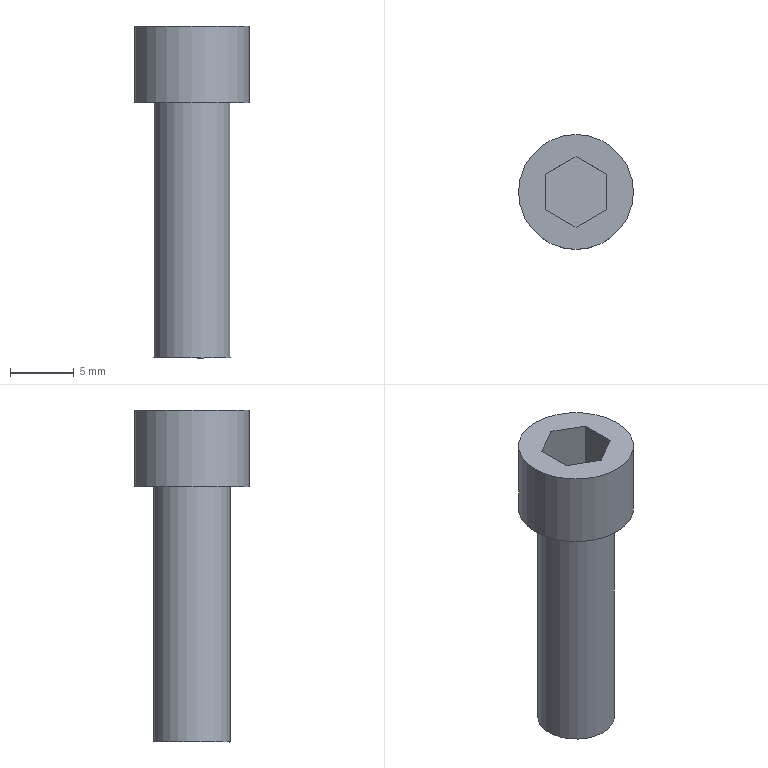Part | NX | features solid 2 | 1 solid | 12 faces | box 9 x 9 x 26 mm | volume 875.359 mm3 | plane 10 | cylinder 2 | commonest cylinder face diameters 6 x1 9 x1
STEP:
#1=CARTESIAN_POINT('',(277.6,-741.386,75.));
#2=VERTEX_POINT('',#1);
#3=CARTESIAN_POINT('',(280.,-742.771,75.));
#4=VERTEX_POINT('',#3);
#5=CARTESIAN_POINT('',(278.8,-742.078,75.));
#6=DIRECTION('',(0.866,-0.5,0.));
#7=VECTOR('',#6,1000.);
#8=LINE('',#5,#7);
#9=EDGE_CURVE('',#2,#4,#8,.T.);
#10=ORIENTED_EDGE('',*,*,#9,.F.);
#11=CARTESIAN_POINT('',(277.6,-738.614,75.));
#12=VERTEX_POINT('',#11);
#13=CARTESIAN_POINT('',(277.6,-740.,75.));
#14=DIRECTION('',(0.,-1.,0.));
#15=VECTOR('',#14,1000.);
#16=LINE('',#13,#15);
#17=EDGE_CURVE('',#12,#2,#16,.T.);
#18=ORIENTED_EDGE('',*,*,#17,.F.);
#19=CARTESIAN_POINT('',(280.,-737.229,75.));
#20=VERTEX_POINT('',#19);
#21=CARTESIAN_POINT('',(278.8,-737.922,75.));
#22=DIRECTION('',(-0.866,-0.5,0.));
#23=VECTOR('',#22,1000.);
#24=LINE('',#21,#23);
#25=EDGE_CURVE('',#20,#12,#24,.T.);
#26=ORIENTED_EDGE('',*,*,#25,.F.);
#27=CARTESIAN_POINT('',(282.4,-738.614,75.));
#28=VERTEX_POINT('',#27);
#29=CARTESIAN_POINT('',(281.2,-737.922,75.));
#30=DIRECTION('',(-0.866,0.5,0.));
#31=VECTOR('',#30,1000.);
#32=LINE('',#29,#31);
#33=EDGE_CURVE('',#28,#20,#32,.T.);
#34=ORIENTED_EDGE('',*,*,#33,.F.);
#35=CARTESIAN_POINT('',(282.4,-741.386,75.));
#36=VERTEX_POINT('',#35);
#37=CARTESIAN_POINT('',(282.4,-740.,75.));
#38=DIRECTION('',(0.,1.,0.));
#39=VECTOR('',#38,1000.);
#40=LINE('',#37,#39);
#41=EDGE_CURVE('',#36,#28,#40,.T.);
#42=ORIENTED_EDGE('',*,*,#41,.F.);
#43=CARTESIAN_POINT('',(281.2,-742.078,75.));
#44=DIRECTION('',(0.866,0.5,0.));
#45=VECTOR('',#44,1000.);
#46=LINE('',#43,#45);
#47=EDGE_CURVE('',#4,#36,#46,.T.);
#48=ORIENTED_EDGE('',*,*,#47,.F.);
#49=EDGE_LOOP('',(#10,#18,#26,#34,#42,#48));
#50=FACE_BOUND('',#49,.T.);
#51=CARTESIAN_POINT('',(280.,-735.5,75.));
#52=VERTEX_POINT('',#51);
#53=CARTESIAN_POINT('',(280.,-740.,75.));
#54=DIRECTION('',(0.,0.,-1.));
#55=DIRECTION('',(0.,1.,0.));
#56=AXIS2_PLACEMENT_3D('',#53,#54,#55);
#57=CIRCLE('',#56,4.5);
#58=EDGE_CURVE('',#52,#52,#57,.T.);
#59=ORIENTED_EDGE('',*,*,#58,.F.);
#60=EDGE_LOOP('',(#59));
#61=FACE_BOUND('',#60,.T.);
#62=CARTESIAN_POINT('',(280.,-740.,75.));
#63=DIRECTION('',(0.,0.,1.));
#64=DIRECTION('',(0.,-1.,0.));
#65=AXIS2_PLACEMENT_3D('',#62,#63,#64);
#66=PLANE('',#65);
#67=ADVANCED_FACE('',(#50,#61),#66,.T.);
#68=CARTESIAN_POINT('',(280.,-737.,69.));
#69=VERTEX_POINT('',#68);
#70=CARTESIAN_POINT('',(280.,-740.,69.));
#71=DIRECTION('',(0.,0.,-1.));
#72=DIRECTION('',(0.,1.,0.));
#73=AXIS2_PLACEMENT_3D('',#70,#71,#72);
#74=CIRCLE('',#73,3.);
#75=EDGE_CURVE('',#69,#69,#74,.T.);
#76=ORIENTED_EDGE('',*,*,#75,.F.);
#77=EDGE_LOOP('',(#76));
#78=FACE_BOUND('',#77,.T.);
#79=CARTESIAN_POINT('',(280.,-744.5,69.));
#80=VERTEX_POINT('',#79);
#81=CARTESIAN_POINT('',(280.,-740.,69.));
#82=DIRECTION('',(0.,0.,1.));
#83=DIRECTION('',(0.,-1.,0.));
#84=AXIS2_PLACEMENT_3D('',#81,#82,#83);
#85=CIRCLE('',#84,4.5);
#86=EDGE_CURVE('',#80,#80,#85,.T.);
#87=ORIENTED_EDGE('',*,*,#86,.F.);
#88=EDGE_LOOP('',(#87));
#89=FACE_BOUND('',#88,.T.);
#90=CARTESIAN_POINT('',(280.,-740.,69.));
#91=DIRECTION('',(0.,0.,-1.));
#92=DIRECTION('',(0.,1.,0.));
#93=AXIS2_PLACEMENT_3D('',#90,#91,#92);
#94=PLANE('',#93);
#95=ADVANCED_FACE('',(#78,#89),#94,.T.);
#96=ORIENTED_EDGE('',*,*,#58,.T.);
#97=EDGE_LOOP('',(#96));
#98=FACE_BOUND('',#97,.T.);
#99=ORIENTED_EDGE('',*,*,#86,.T.);
#100=EDGE_LOOP('',(#99));
#101=FACE_BOUND('',#100,.T.);
#102=CARTESIAN_POINT('',(280.,-740.,69.));
#103=DIRECTION('',(0.,0.,1.));
#104=DIRECTION('',(0.,-1.,0.));
#105=AXIS2_PLACEMENT_3D('',#102,#103,#104);
#106=CYLINDRICAL_SURFACE('',#105,4.5);
#107=ADVANCED_FACE('',(#98,#101),#106,.T.);
#108=ORIENTED_EDGE('',*,*,#9,.T.);
#109=CARTESIAN_POINT('',(280.,-742.771,71.4));
#110=VERTEX_POINT('',#109);
#111=CARTESIAN_POINT('',(280.,-742.771,71.4));
#112=DIRECTION('',(0.,0.,1.));
#113=VECTOR('',#112,1000.);
#114=LINE('',#111,#113);
#115=EDGE_CURVE('',#110,#4,#114,.T.);
#116=ORIENTED_EDGE('',*,*,#115,.F.);
#117=CARTESIAN_POINT('',(277.6,-741.386,71.4));
#118=VERTEX_POINT('',#117);
#119=CARTESIAN_POINT('',(277.6,-741.386,71.4));
#120=DIRECTION('',(0.866,-0.5,0.));
#121=VECTOR('',#120,1000.);
#122=LINE('',#119,#121);
#123=EDGE_CURVE('',#118,#110,#122,.T.);
#124=ORIENTED_EDGE('',*,*,#123,.F.);
#125=CARTESIAN_POINT('',(277.6,-741.386,71.4));
#126=DIRECTION('',(0.,0.,1.));
#127=VECTOR('',#126,1000.);
#128=LINE('',#125,#127);
#129=EDGE_CURVE('',#118,#2,#128,.T.);
#130=ORIENTED_EDGE('',*,*,#129,.T.);
#131=EDGE_LOOP('',(#108,#116,#124,#130));
#132=FACE_BOUND('',#131,.T.);
#133=CARTESIAN_POINT('',(278.8,-742.078,74.4));
#134=DIRECTION('',(-0.5,-0.866,0.));
#135=DIRECTION('',(0.866,-0.5,0.));
#136=AXIS2_PLACEMENT_3D('',#133,#134,#135);
#137=PLANE('',#136);
#138=ADVANCED_FACE('',(#132),#137,.F.);
#139=ORIENTED_EDGE('',*,*,#17,.T.);
#140=ORIENTED_EDGE('',*,*,#129,.F.);
#141=CARTESIAN_POINT('',(277.6,-738.614,71.4));
#142=VERTEX_POINT('',#141);
#143=CARTESIAN_POINT('',(277.6,-738.614,71.4));
#144=DIRECTION('',(0.,-1.,0.));
#145=VECTOR('',#144,1000.);
#146=LINE('',#143,#145);
#147=EDGE_CURVE('',#142,#118,#146,.T.);
#148=ORIENTED_EDGE('',*,*,#147,.F.);
#149=CARTESIAN_POINT('',(277.6,-738.614,71.4));
#150=DIRECTION('',(0.,0.,1.));
#151=VECTOR('',#150,1000.);
#152=LINE('',#149,#151);
#153=EDGE_CURVE('',#142,#12,#152,.T.);
#154=ORIENTED_EDGE('',*,*,#153,.T.);
#155=EDGE_LOOP('',(#139,#140,#148,#154));
#156=FACE_BOUND('',#155,.T.);
#157=CARTESIAN_POINT('',(277.6,-740.,74.4));
#158=DIRECTION('',(-1.,0.,0.));
#159=DIRECTION('',(0.,-1.,0.));
#160=AXIS2_PLACEMENT_3D('',#157,#158,#159);
#161=PLANE('',#160);
#162=ADVANCED_FACE('',(#156),#161,.F.);
#163=ORIENTED_EDGE('',*,*,#25,.T.);
#164=ORIENTED_EDGE('',*,*,#153,.F.);
#165=CARTESIAN_POINT('',(280.,-737.229,71.4));
#166=VERTEX_POINT('',#165);
#167=CARTESIAN_POINT('',(280.,-737.229,71.4));
#168=DIRECTION('',(-0.866,-0.5,0.));
#169=VECTOR('',#168,1000.);
#170=LINE('',#167,#169);
#171=EDGE_CURVE('',#166,#142,#170,.T.);
#172=ORIENTED_EDGE('',*,*,#171,.F.);
#173=CARTESIAN_POINT('',(280.,-737.229,71.4));
#174=DIRECTION('',(0.,0.,1.));
#175=VECTOR('',#174,1000.);
#176=LINE('',#173,#175);
#177=EDGE_CURVE('',#166,#20,#176,.T.);
#178=ORIENTED_EDGE('',*,*,#177,.T.);
#179=EDGE_LOOP('',(#163,#164,#172,#178));
#180=FACE_BOUND('',#179,.T.);
#181=CARTESIAN_POINT('',(278.8,-737.922,74.4));
#182=DIRECTION('',(-0.5,0.866,0.));
#183=DIRECTION('',(-0.866,-0.5,0.));
#184=AXIS2_PLACEMENT_3D('',#181,#182,#183);
#185=PLANE('',#184);
#186=ADVANCED_FACE('',(#180),#185,.F.);
#187=ORIENTED_EDGE('',*,*,#33,.T.);
#188=ORIENTED_EDGE('',*,*,#177,.F.);
#189=CARTESIAN_POINT('',(282.4,-738.614,71.4));
#190=VERTEX_POINT('',#189);
#191=CARTESIAN_POINT('',(282.4,-738.614,71.4));
#192=DIRECTION('',(-0.866,0.5,0.));
#193=VECTOR('',#192,1000.);
#194=LINE('',#191,#193);
#195=EDGE_CURVE('',#190,#166,#194,.T.);
#196=ORIENTED_EDGE('',*,*,#195,.F.);
#197=CARTESIAN_POINT('',(282.4,-738.614,71.4));
#198=DIRECTION('',(0.,0.,1.));
#199=VECTOR('',#198,1000.);
#200=LINE('',#197,#199);
#201=EDGE_CURVE('',#190,#28,#200,.T.);
#202=ORIENTED_EDGE('',*,*,#201,.T.);
#203=EDGE_LOOP('',(#187,#188,#196,#202));
#204=FACE_BOUND('',#203,.T.);
#205=CARTESIAN_POINT('',(281.2,-737.922,74.4));
#206=DIRECTION('',(0.5,0.866,0.));
#207=DIRECTION('',(-0.866,0.5,0.));
#208=AXIS2_PLACEMENT_3D('',#205,#206,#207);
#209=PLANE('',#208);
#210=ADVANCED_FACE('',(#204),#209,.F.);
#211=ORIENTED_EDGE('',*,*,#41,.T.);
#212=ORIENTED_EDGE('',*,*,#201,.F.);
#213=CARTESIAN_POINT('',(282.4,-741.386,71.4));
#214=VERTEX_POINT('',#213);
#215=CARTESIAN_POINT('',(282.4,-741.386,71.4));
#216=DIRECTION('',(0.,1.,0.));
#217=VECTOR('',#216,1000.);
#218=LINE('',#215,#217);
#219=EDGE_CURVE('',#214,#190,#218,.T.);
#220=ORIENTED_EDGE('',*,*,#219,.F.);
#221=CARTESIAN_POINT('',(282.4,-741.386,71.4));
#222=DIRECTION('',(0.,0.,1.));
#223=VECTOR('',#222,1000.);
#224=LINE('',#221,#223);
#225=EDGE_CURVE('',#214,#36,#224,.T.);
#226=ORIENTED_EDGE('',*,*,#225,.T.);
#227=EDGE_LOOP('',(#211,#212,#220,#226));
#228=FACE_BOUND('',#227,.T.);
#229=CARTESIAN_POINT('',(282.4,-740.,74.4));
#230=DIRECTION('',(1.,0.,0.));
#231=DIRECTION('',(0.,1.,0.));
#232=AXIS2_PLACEMENT_3D('',#229,#230,#231);
#233=PLANE('',#232);
#234=ADVANCED_FACE('',(#228),#233,.F.);
#235=ORIENTED_EDGE('',*,*,#47,.T.);
#236=ORIENTED_EDGE('',*,*,#225,.F.);
#237=CARTESIAN_POINT('',(280.,-742.771,71.4));
#238=DIRECTION('',(0.866,0.5,0.));
#239=VECTOR('',#238,1000.);
#240=LINE('',#237,#239);
#241=EDGE_CURVE('',#110,#214,#240,.T.);
#242=ORIENTED_EDGE('',*,*,#241,.F.);
#243=ORIENTED_EDGE('',*,*,#115,.T.);
#244=EDGE_LOOP('',(#235,#236,#242,#243));
#245=FACE_BOUND('',#244,.T.);
#246=CARTESIAN_POINT('',(281.2,-742.078,74.4));
#247=DIRECTION('',(0.5,-0.866,0.));
#248=DIRECTION('',(0.866,0.5,0.));
#249=AXIS2_PLACEMENT_3D('',#246,#247,#248);
#250=PLANE('',#249);
#251=ADVANCED_FACE('',(#245),#250,.F.);
#252=ORIENTED_EDGE('',*,*,#241,.T.);
#253=ORIENTED_EDGE('',*,*,#219,.T.);
#254=ORIENTED_EDGE('',*,*,#195,.T.);
#255=ORIENTED_EDGE('',*,*,#171,.T.);
#256=ORIENTED_EDGE('',*,*,#147,.T.);
#257=ORIENTED_EDGE('',*,*,#123,.T.);
#258=EDGE_LOOP('',(#252,#253,#254,#255,#256,#257));
#259=FACE_BOUND('',#258,.T.);
#260=CARTESIAN_POINT('',(280.,-740.,71.4));
#261=DIRECTION('',(0.,0.,-1.));
#262=DIRECTION('',(0.,1.,0.));
#263=AXIS2_PLACEMENT_3D('',#260,#261,#262);
#264=PLANE('',#263);
#265=ADVANCED_FACE('',(#259),#264,.F.);
#266=CARTESIAN_POINT('',(280.,-743.,49.));
#267=VERTEX_POINT('',#266);
#268=CARTESIAN_POINT('',(280.,-740.,49.));
#269=DIRECTION('',(0.,0.,1.));
#270=DIRECTION('',(0.,-1.,0.));
#271=AXIS2_PLACEMENT_3D('',#268,#269,#270);
#272=CIRCLE('',#271,3.);
#273=EDGE_CURVE('',#267,#267,#272,.T.);
#274=ORIENTED_EDGE('',*,*,#273,.F.);
#275=EDGE_LOOP('',(#274));
#276=FACE_BOUND('',#275,.T.);
#277=CARTESIAN_POINT('',(280.,-740.,49.));
#278=DIRECTION('',(0.,0.,-1.));
#279=DIRECTION('',(0.,1.,0.));
#280=AXIS2_PLACEMENT_3D('',#277,#278,#279);
#281=PLANE('',#280);
#282=ADVANCED_FACE('',(#276),#281,.T.);
#283=ORIENTED_EDGE('',*,*,#273,.T.);
#284=EDGE_LOOP('',(#283));
#285=FACE_BOUND('',#284,.T.);
#286=ORIENTED_EDGE('',*,*,#75,.T.);
#287=EDGE_LOOP('',(#286));
#288=FACE_BOUND('',#287,.T.);
#289=CARTESIAN_POINT('',(280.,-740.,69.));
#290=DIRECTION('',(0.,0.,-1.));
#291=DIRECTION('',(0.,1.,0.));
#292=AXIS2_PLACEMENT_3D('',#289,#290,#291);
#293=CYLINDRICAL_SURFACE('',#292,3.);
#294=ADVANCED_FACE('',(#285,#288),#293,.T.);
#295=CLOSED_SHELL('',(#67,#95,#107,#138,#162,#186,#210,#234,#251,#265,#282,#294));
#296=MANIFOLD_SOLID_BREP('',#295);
#297=(LENGTH_UNIT()NAMED_UNIT(*)SI_UNIT(.MILLI.,.METRE.));
#298=UNCERTAINTY_MEASURE_WITH_UNIT(LENGTH_MEASURE(0.00001),#297,'','');
#299=(NAMED_UNIT(*)PLANE_ANGLE_UNIT()SI_UNIT($,.RADIAN.));
#300=(NAMED_UNIT(*)SI_UNIT($,.STERADIAN.)SOLID_ANGLE_UNIT());
#301=(GEOMETRIC_REPRESENTATION_CONTEXT(3)GLOBAL_UNCERTAINTY_ASSIGNED_CONTEXT((#298))GLOBAL_UNIT_ASSIGNED_CONTEXT((#297,#299,#300))REPRESENTATION_CONTEXT('',''));
#302=ADVANCED_BREP_SHAPE_REPRESENTATION('',(#296),#301);